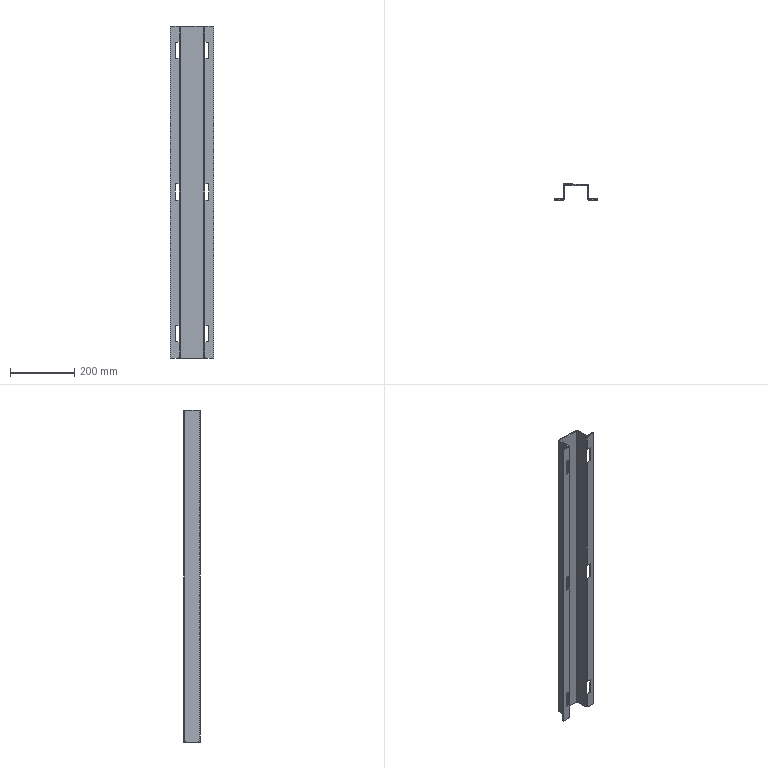Part | STEP file | TS-020-01 | 1 solid | 102 faces | box 134 x 49.886 x 1030 mm | volume 673543 mm3 | plane 58 | cylinder 36 | spline 8 | commonest cylinder face diameters 6 x16 0.4 x10 6.4 x10